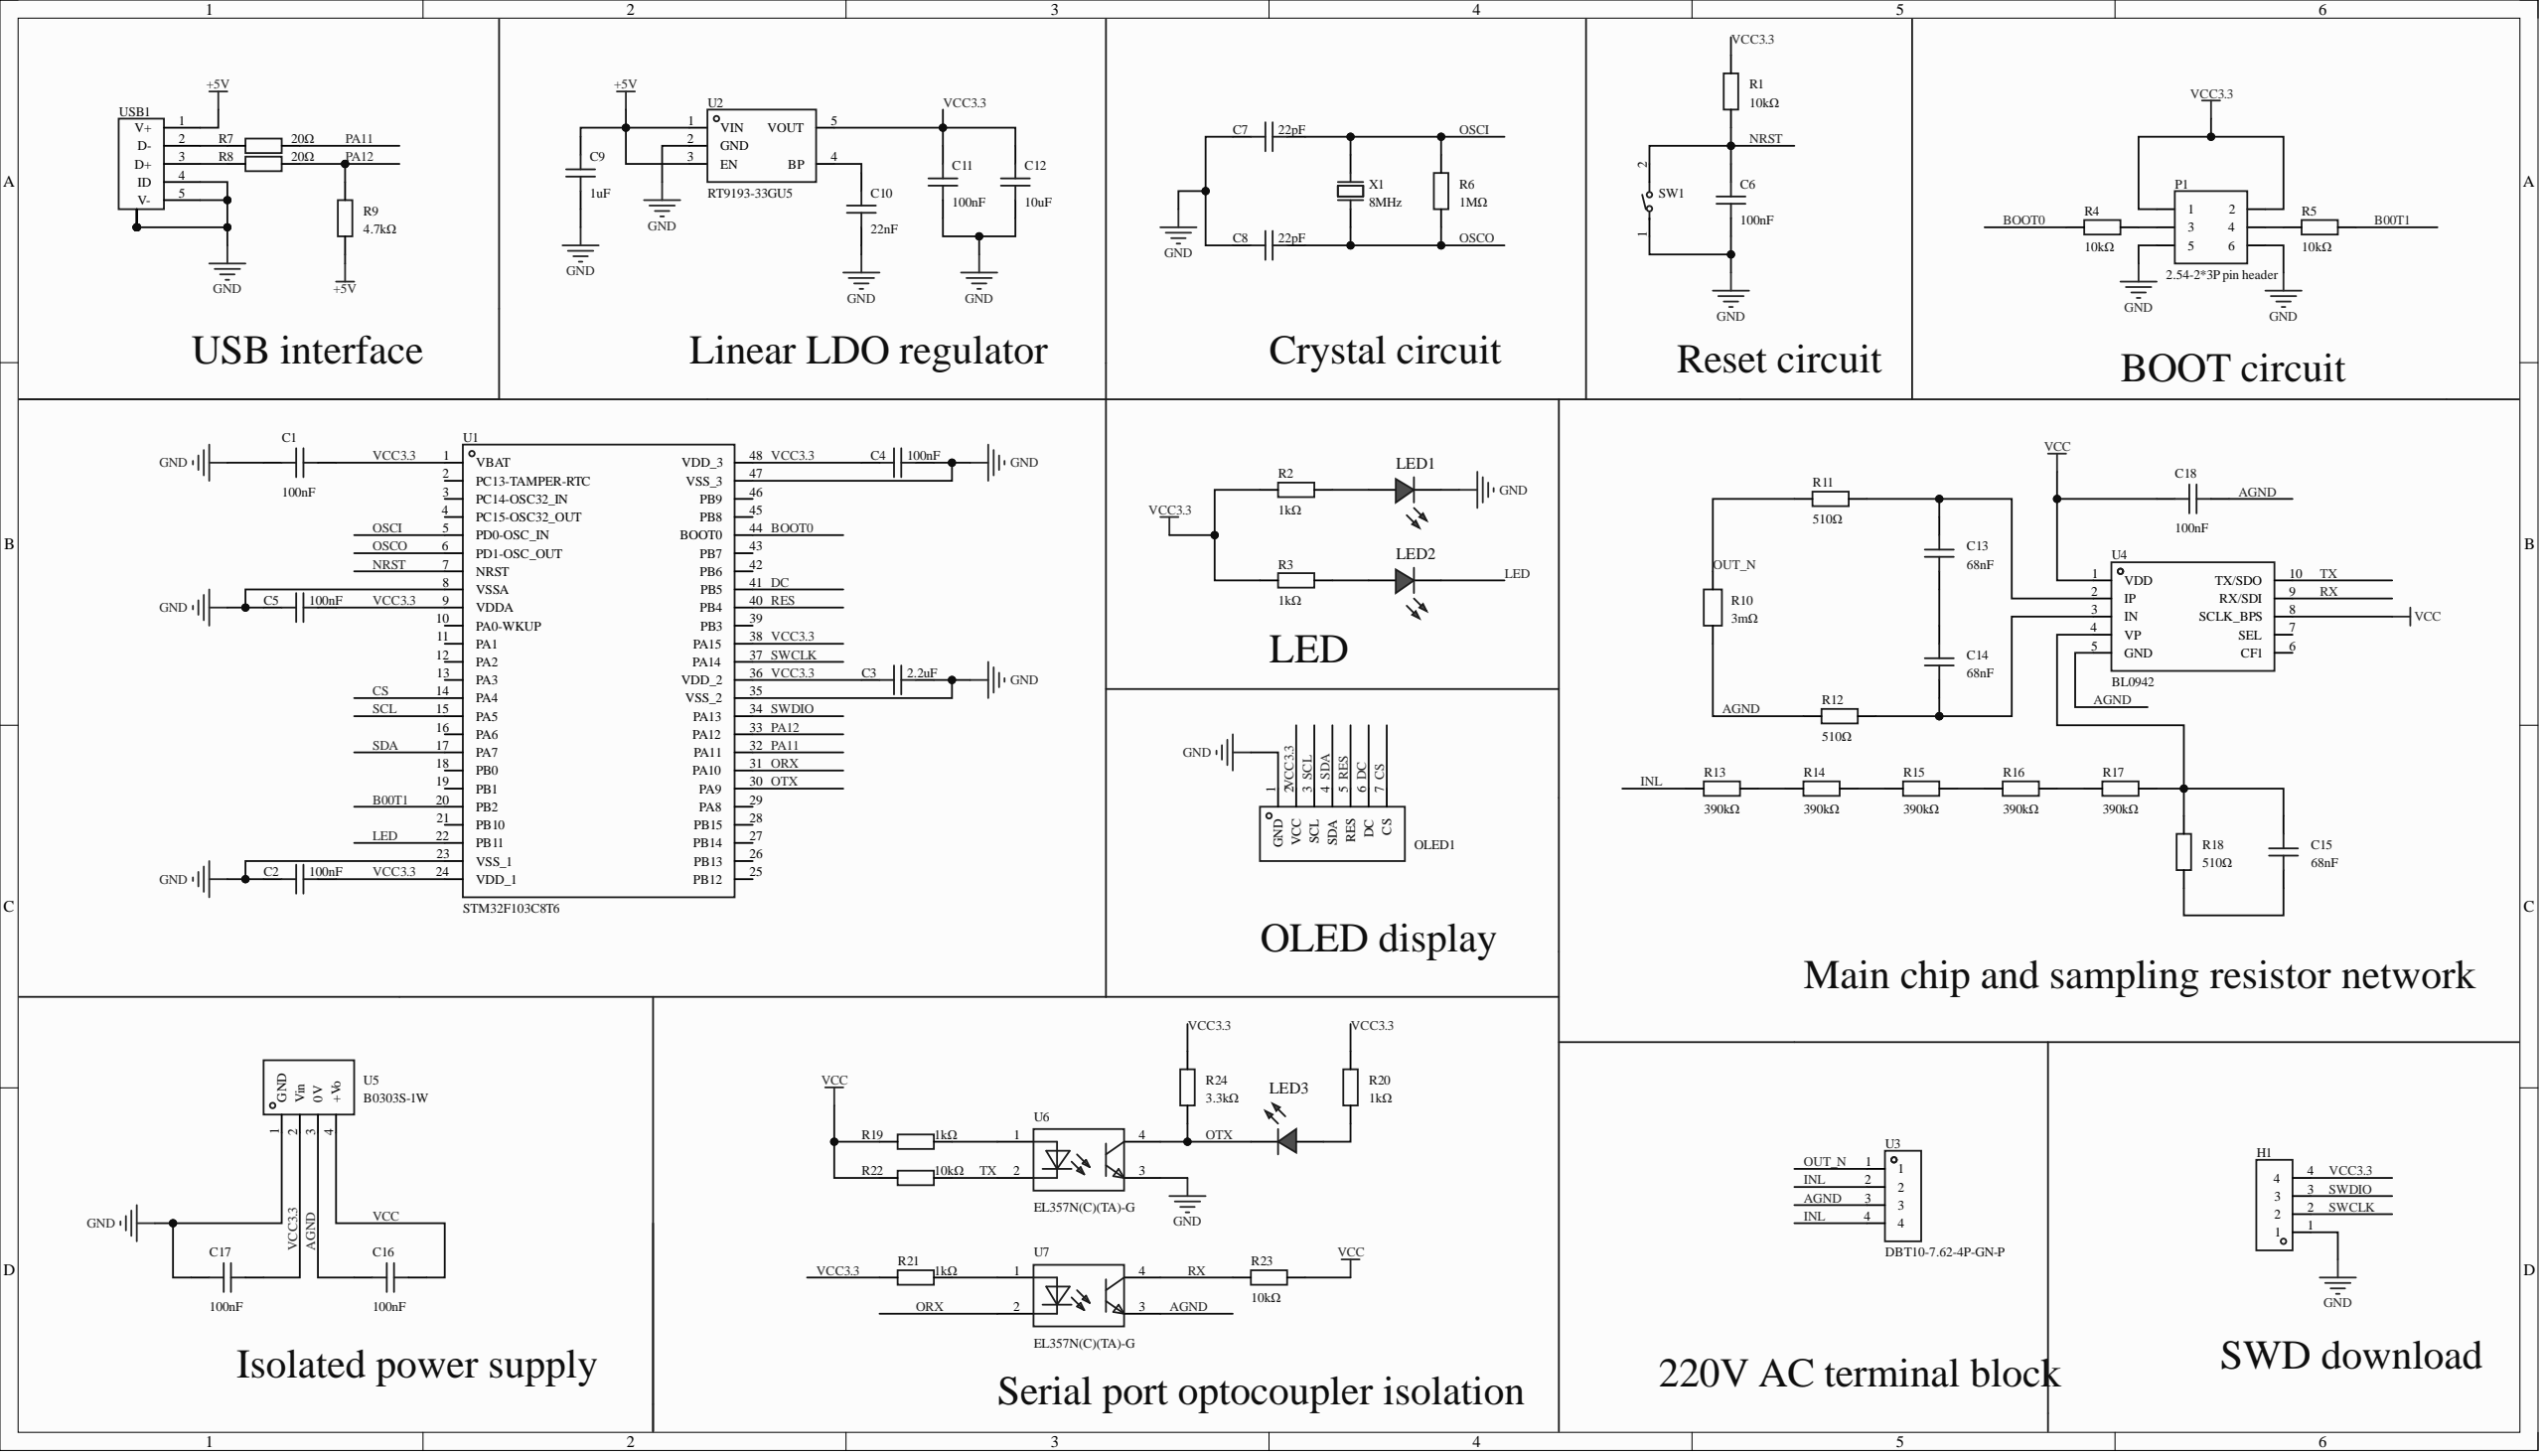Circuit board | Altium Designer | 62 parts | 45 nets
Bill of materials:
Comment,Description,Designator,Footprint,LibRef,Quantity
"100nF","Capacitance: 100nF;Tolerance: ±10%;Rated voltage: 50V;Temperature coefficient: X7R;","C1, C2, C4, C5, C6, C11, C16, C17, C18","CAP-SMD_L2.0-W1.25","FCC0805B104K500DT","9"
"2.2uF","","C3","C0805","CAP_0805","1"
"22pF","","C7, C8","C0805","CAP_0805","2"
"1uF","","C9","C0805","CAP_0805","1"
"22nF","","C10","C0805","CAP_0805","1"
"10uF","","C12","C0805","CAP_0805","1"
"68nF","","C13, C14, C15","C0805","CAP_0805","3"
"PZ254V-11-04P","插针结构:1x4P;间距:2.54mm;行距:-;圆针/方针:方针;安装方式:直插;排数:单排;总PIN位数:4P;额定电流:3A;额定电压:250V;配合针长度:6mm;塑高:2.5mm;端接针长度:3mm;触头材质:-;工作温度:-40℃~+105℃;颜色:黑色;","H1","HDR-TH_4P-P2.54-V-M","PZ254V-11-04P","1"
"","","LED1, LED2, LED3","LED_0805","LED_0805-R","3"
"HS96L01W4S03","Size (inch): 0.96;Pixel resolution: 128x64;","OLED1","OLED-TH_HS96L01W4S03","HS96L01W4S03","1"
"2.54-2*3P pin header","连接器类型:简牛座;间距:2.54mm;结构:2x3P;额定电流:1A;安装方式:直插;行距:2.54mm;排数:2;每排PIN数:3;触头材质:黄铜;触头镀层:金;工作温度:-55℃~+105℃;","P1","IDC-TH_6P-P2.54_C11214","2.54-2*3P简牛","1"
"10kΩ","","R1, R4, R5, R22, R23","R0805","Res_0805","5"
"1kΩ","","R2, R3, R19, R20, R21","R0805","Res_0805","5"
"1MΩ","","R6","R0805","Res_0805","1"
"20Ω","","R7, R8","R0805","Res_0805","2"
"4.7kΩ","","R9","R0805","Res_0805","1"
"3mΩ","Resistor type: sampling resistor; alloy resistor;Resistance: 3mΩ;Tolerance: ±1%;Power: 3W;Temperature coefficient: ±50ppm/?;","R10","R2512","JER2512F3R003L","1"
"510Ω","","R11, R12, R18","R0805","Res_0805","3"
"390kΩ","","R13, R14, R15, R16, R17","R0805","Res_0805","5"
"3.3kΩ","","R24","R0805","Res_0805","1"
"","","SCREW1, SCREW2, SCREW3, SCREW4","M3螺丝","M3螺丝","4"
"TS1305-TZ43HBM","电路结构:单刀单掷;按钮形状:矩形按钮;安装方式:立贴;开关长度:6mm;开关宽度:3.5mm;开关高度:4.3mm;带支架:不带支架;触点电流:50mA;额定电压:12V;带灯:无;","SW1","SW-SMD_L6.0-W3.5-LS8.0_TS04-TBW1FH4.3","TS1305-TZ43HBM","1"
"STM32F103C8T6","CPU core: ARM-M3;CPU max frequency: 72MHz;Application field: -;","U1","LQFP-48_L7.0-W7.0-P0.50-LS9.0-BL","STM32F103C8T6","1"
"RT9193-33GU5","Output type: fixed;Operating voltage: 5.5V;Output voltage: 3.3V;Output current: 300mA;PSRR: 70dB@(100Hz);Output polarity: positive;","U2","SC-70-5_L2.0-W1.3-P0.65-LS2.1-BL","RT9193-33GU5","1"
"DBT10-7.62-4P-GN-P","隔板类型:两面;间距:7.62mm;结构:1x4P;安装方式:直插;引脚位置:边脚;排数:1;每排PIN数:4;额定电流:24A;额定电压:450V;线规 - AWG:14~22;线规 - 平方毫米:-;工作温度:-40℃~+105℃;颜色:绿色;","U3","CONN-TH_DBT10-7.62-4P","DBT10-7.62-4P-GN-P","1"
"BL0942","BL0942 is an energy metering chip with built-in clock and no calibration required, suitable for single-phase multifunction energy meters, smart sockets, smart home appliances and similar applications, with high cost-effectiveness.","U4","SSOP-10_L4.9-W3.9-P1.00-LS6.0-BL","BL0942_C2837510","1"
"B0303S-1W","Size (mm): length 11.6 * width 6.0 * height 10.0","U5","PWRM-TH_BXXXXS-1W","B0303S-1W_C5280457","1"
"EL357N(C)(TA)-G","输入类型:DC;正向压降(Vf):1.2V;输出电流:50mA;隔离电压(Vrms):3.75kV;直流反向耐压(Vr):6V;负载电压:80V;输出通道数:1;集射极饱和电压(VCE(sat)):200mV@20mA,1mA;","U6, U7","OPTO-SMD-4_L4.4-W4.1-P2.54-LS7.0-TL","EL357N(C)(TA)-G_C42379244","2"
"920-E52A2021S10100","Connector type: Micro-B;Protocol standard: USB 2.0;Gender: female;Mounting: horizontal SMD;Contacts: 5P;Ports: 1;Rated current - power: 1A;Operating temperature: -30℃~+80℃;","USB1","MICRO-USB-SMD_5P-P0.65-H-F_C10418","920-E52A2021S10100","1"
"8MHz","Crystal type: SMD crystal;Frequency: 8MHz;Frequency deviation at room temperature: ±30ppm;Load capacitance: 20pF;Frequency stability: ±50ppm;","X1","CRYSTAL-SMD_L11.4-W4.7-LS12.7","X49SS2-8.000-F20JGDT","1"
Netlist (Protel format):
[
C1
CAP-SMD_L2.0-W1.25
100nF



]
[
C2
CAP-SMD_L2.0-W1.25
100nF



]
[
C3
C0805
2.2uF



]
[
C4
CAP-SMD_L2.0-W1.25
100nF



]
[
C5
CAP-SMD_L2.0-W1.25
100nF



]
[
C6
CAP-SMD_L2.0-W1.25
100nF



]
[
C7
C0805
22pF



]
[
C8
C0805
22pF



]
[
C9
C0805
1uF



]
[
C10
C0805
22nF



]
[
C11
CAP-SMD_L2.0-W1.25
100nF



]
[
C12
C0805
10uF



]
[
C13
C0805
68nF



]
[
C14
C0805
68nF



]
[
C15
C0805
68nF



]
[
C16
CAP-SMD_L2.0-W1.25
100nF



]
[
C17
CAP-SMD_L2.0-W1.25
100nF



]
[
C18
CAP-SMD_L2.0-W1.25
100nF



]
[
H1
HDR-TH_4P-P2.54-V-M
PZ254V-11-04P



]
[
LED1
LED_0805




]
[
LED2
LED_0805




]
[
LED3
LED_0805




]
[
OLED1
OLED-TH_HS96L01W4S03
HS96L01W4S03



]
[
P1
IDC-TH_6P-P2.54_C11214
2.54-2*3P pin header



]
[
R1
R0805
10kΩ



]
[
R2
R0805
1kΩ



]
[
R3
R0805
1kΩ



]
[
R4
R0805
10kΩ



]
[
R5
R0805
10kΩ



]
[
R6
R0805
1MΩ



]
[
R7
R0805
20Ω



]
[
R8
R0805
20Ω



]
[
R9
R0805
4.7kΩ



]
[
R10
R2512
3mΩ



]
[
R11
R0805
510Ω



]
[
R12
R0805
510Ω



]
[
R13
R0805
390kΩ



]
[
R14
R0805
390kΩ



]
[
R15
R0805
390kΩ



]
[
R16
R0805
390kΩ



]
[
R17
R0805
390kΩ



]
[
R18
R0805
510Ω



]
[
R19
R0805
1kΩ



]
[
R20
R0805
1kΩ



]
[
R21
R0805
1kΩ



]
[
R22
R0805
10kΩ



]
[
R23
R0805
10kΩ



]
[
R24
R0805
3.3kΩ



]
[
SCREW1
M3螺丝




]
[
SCREW2
M3螺丝




]
[
SCREW3
M3螺丝




]
[
SCREW4
M3螺丝




]
[
SW1
SW-SMD_L6.0-W3.5-LS8.0_TS04-TBW1FH4.3
TS1305-TZ43HBM



]
[
U1
LQFP-48_L7.0-W7.0-P0.50-LS9.0-BL
STM32F103C8T6



]
[
U2
SC-70-5_L2.0-W1.3-P0.65-LS2.1-BL
RT9193-33GU5



]
[
U3
CONN-TH_DBT10-7.62-4P
DBT10-7.62-4P-GN-P



]
[
U4
SSOP-10_L4.9-W3.9-P1.00-LS6.0-BL
BL0942



]
[
U5
PWRM-TH_BXXXXS-1W
B0303S-1W



]
[
U6
OPTO-SMD-4_L4.4-W4.1-P2.54-LS7.0-TL
EL357N(C)(TA)-G



]
[
U7
OPTO-SMD-4_L4.4-W4.1-P2.54-LS7.0-TL
EL357N(C)(TA)-G



]
[
USB1
MICRO-USB-SMD_5P-P0.65-H-F_C10418
920-E52A2021S10100



]
[
X1
CRYSTAL-SMD_L11.4-W4.7-LS12.7
8MHz



]
(
VCC3.3
C1-2
C2-2
C3-1
C4-2
C5-2
C11-1
C12-2
C17-2
H1-4
OLED1-2
P1-1
P1-2
R1-2
R2-2
R3-2
R20-1
R21-2
R24-1
U1-1
U1-9
U1-24
U1-36
U1-38
U1-48
U2-5
U5-2
)
(
VCC
C16-2
C18-1
R19-2
R22-2
R23-2
U4-1
U4-8
U5-4
)
(
TX
R22-1
U4-10
U6-2
)
(
SWDIO
H1-3
U1-34
)
(
SWCLK
H1-2
U1-37
)
(
SDA
OLED1-4
U1-17
)
(
SCL
OLED1-3
U1-15
)
(
RX
R23-1
U4-9
U7-4
)
(
RES
OLED1-5
U1-40
)
(
PA12
R8-2
R9-2
U1-33
)
(
PA11
R7-2
U1-32
)
(
OUT_N
R10-2
R11-2
U3-1
)
(
OTX
LED3-1
R24-2
U1-30
U6-4
)
(
OSCO
C8-1
R6-1
U1-6
X1-1
)
(
OSCI
C7-1
R6-2
U1-5
X1-2
)
(
ORX
U1-31
U7-2
)
(
NRST
C6-1
R1-1
SW1-2
U1-7
)
(
NetR21_1
R21-1
U7-1
)
(
NetR19_1
R19-1
U6-1
)
(
NetR16_1
R16-1
R17-2
)
(
NetR15_1
R15-1
R16-2
)
(
NetR14_1
R14-1
R15-2
)
(
NetR13_1
R13-1
R14-2
)
(
NetR8_1
R8-1
USB1-3
)
(
NetR7_1
R7-1
USB1-2
)
(
NetP1_4
P1-4
R5-2
)
(
NetP1_3
P1-3
R4-1
)
(
NetLED3_2
LED3-2
R20-2
)
(
NetLED2_2
LED2-2
R3-1
)
(
NetLED1_2
LED1-2
R2-1
)
(
NetC15_2
C15-2
R18-2
)
(
NetC15_1
C15-1
R17-1
R18-1
U4-4
)
(
NetC14_2
C14-2
R12-1
U4-3
)
(
NetC13_2
C13-2
C14-1
)
(
NetC13_1
C13-1
R11-1
U4-2
)
(
NetC10_2
C10-2
U2-4
)
(
LED
LED2-1
U1-22
)
(
INL
R13-2
U3-2
U3-4
)
(
GND
C1-1
C2-1
C3-2
C4-1
C5-1
C6-2
C7-2
C8-2
C9-1
C10-1
C11-2
C12-1
C17-1
H1-1
LED1-1
OLED1-1
P1-5
P1-6
SW1-1
U1-8
U1-23
U1-35
U1-47
U2-2
U5-1
U6-3
USB1-4
USB1-5
USB1-SH0
USB1-SH1
USB1-SH2
USB1-SH3
)
(
DC
OLED1-6
U1-41
)
(
CS
OLED1-7
U1-14
)
(
BOOT0
R4-2
U1-44
)
(
B00T1
R5-1
U1-20
)
(
AGND
C16-1
C18-2
R10-1
R12-2
U3-3
U4-5
U5-3
U7-3
)
(
+5V
C9-2
R9-1
U2-1
U2-3
USB1-1
)